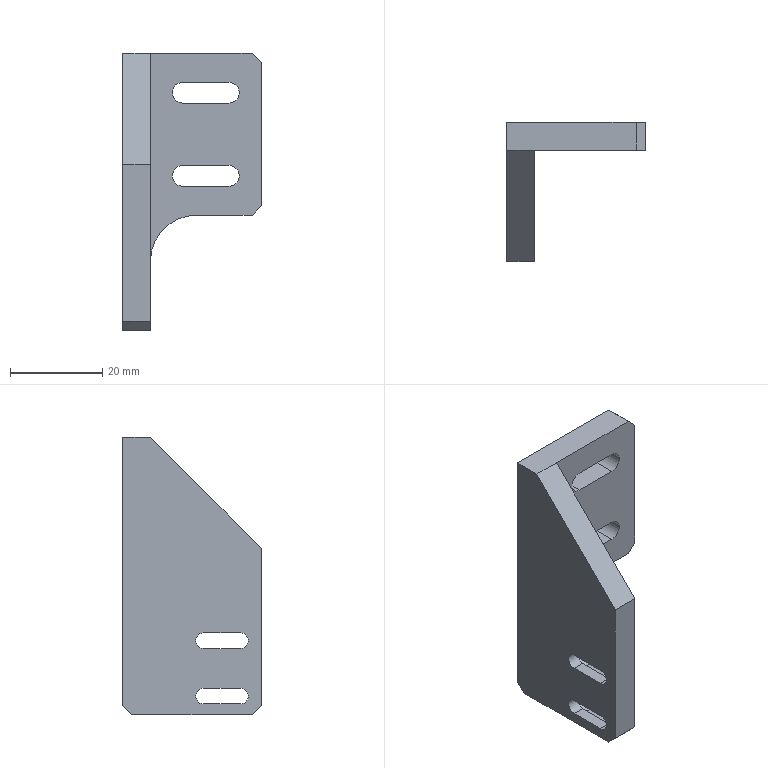Part | STEP file | 0-19-02 Finger cylinder mounting plate | 1 solid | 41 faces | box 30 x 30 x 60 mm | volume 12755 mm3 | plane 28 | cylinder 13 | commonest cylinder face diameters 3.4 x4 4.5 x4 6 x4 20 x1